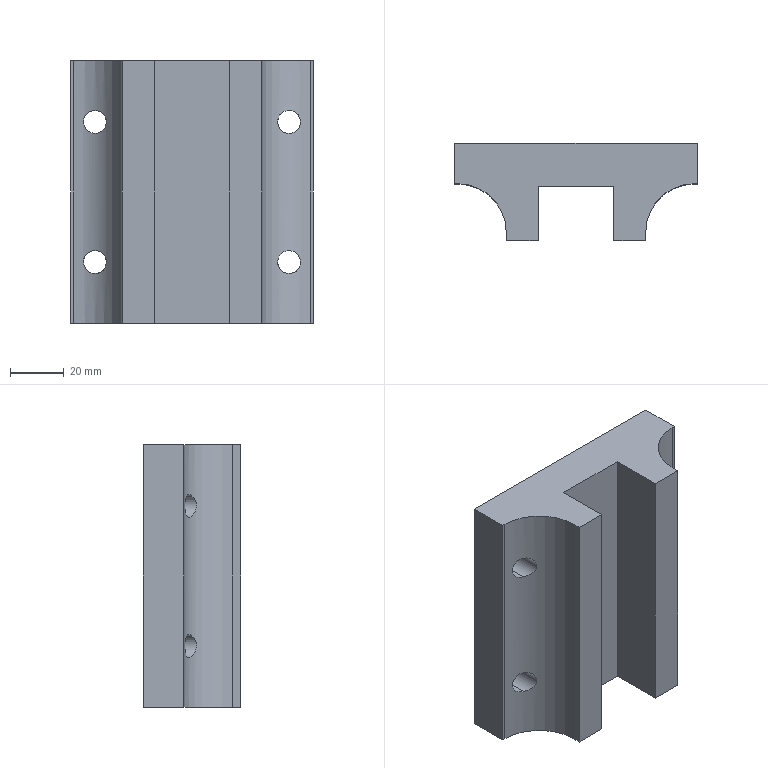Part | SolidWorks | features Extrusion 1, HoleWzd 1 | 1 solid | 24 faces | box 90 x 36 x 97.4 mm | volume 192306 mm3 | plane 14 | cylinder 10 | commonest cylinder face diameters 8.5 x8 36 x2
STEP:
#1=CARTESIAN_POINT('',(36.,-16.792,21.75));
#2=VERTEX_POINT('',#1);
#3=CARTESIAN_POINT('',(36.,-16.792,30.25));
#4=VERTEX_POINT('',#3);
#5=CARTESIAN_POINT('',(36.,-16.792,21.75));
#6=CARTESIAN_POINT('',(35.726,-16.925,21.75));
#7=CARTESIAN_POINT('',(35.454,-17.065,21.776));
#8=CARTESIAN_POINT('',(34.923,-17.356,21.88));
#9=CARTESIAN_POINT('',(34.668,-17.504,21.956));
#10=CARTESIAN_POINT('',(34.176,-17.805,22.152));
#11=CARTESIAN_POINT('',(33.939,-17.959,22.274));
#12=CARTESIAN_POINT('',(33.491,-18.263,22.559));
#13=CARTESIAN_POINT('',(33.282,-18.413,22.722));
#14=CARTESIAN_POINT('',(32.893,-18.702,23.088));
#15=CARTESIAN_POINT('',(32.712,-18.843,23.293));
#16=CARTESIAN_POINT('',(32.388,-19.104,23.744));
#17=CARTESIAN_POINT('',(32.246,-19.222,23.986));
#18=CARTESIAN_POINT('',(32.009,-19.425,24.512));
#19=CARTESIAN_POINT('',(31.913,-19.51,24.796));
#20=CARTESIAN_POINT('',(31.785,-19.624,25.381));
#21=CARTESIAN_POINT('',(31.75,-19.656,25.691));
#22=CARTESIAN_POINT('',(31.75,-19.656,26.148));
#23=CARTESIAN_POINT('',(31.758,-19.649,26.3));
#24=CARTESIAN_POINT('',(31.79,-19.62,26.602));
#25=CARTESIAN_POINT('',(31.815,-19.598,26.754));
#26=CARTESIAN_POINT('',(31.911,-19.512,27.197));
#27=CARTESIAN_POINT('',(32.004,-19.429,27.476));
#28=CARTESIAN_POINT('',(32.243,-19.225,28.008));
#29=CARTESIAN_POINT('',(32.384,-19.107,28.251));
#30=CARTESIAN_POINT('',(32.705,-18.848,28.699));
#31=CARTESIAN_POINT('',(32.887,-18.706,28.906));
#32=CARTESIAN_POINT('',(33.279,-18.415,29.275));
#33=CARTESIAN_POINT('',(33.488,-18.265,29.439));
#34=CARTESIAN_POINT('',(33.936,-17.961,29.725));
#35=CARTESIAN_POINT('',(34.174,-17.806,29.847));
#36=CARTESIAN_POINT('',(34.665,-17.505,30.044));
#37=CARTESIAN_POINT('',(34.92,-17.357,30.119));
#38=CARTESIAN_POINT('',(35.448,-17.068,30.223));
#39=CARTESIAN_POINT('',(35.723,-16.926,30.25));
#40=CARTESIAN_POINT('',(36.,-16.792,30.25));
#41=B_SPLINE_CURVE_WITH_KNOTS('',3,(#5,#6,#7,#8,#9,#10,#11,#12,#13,#14,#15,#16,#17,#18,#19,#20,#21,#22,#23,#24,#25,#26,#27,#28,#29,#30,#31,#32,#33,#34,#35,#36,#37,#38,#39,#40),.UNSPECIFIED.,.F.,.F.,(4,2,2,2,2,2,2,2,2,2,2,2,2,2,2,2,2,4),(0.01371,0.01462,0.01554,0.01645,0.01736,0.01827,0.01918,0.02009,0.02101,0.02146,0.02192,0.02283,0.02374,0.02465,0.02557,0.02648,0.02739,0.0283),.UNSPECIFIED.);
#42=EDGE_CURVE('',#2,#4,#41,.T.);
#43=ORIENTED_EDGE('',*,*,#42,.F.);
#44=CARTESIAN_POINT('',(36.,0.,21.75));
#45=VERTEX_POINT('',#44);
#46=CARTESIAN_POINT('',(36.,0.,21.75));
#47=DIRECTION('',(0.,1.,0.));
#48=VECTOR('',#47,1000.);
#49=LINE('',#46,#48);
#50=EDGE_CURVE('',#2,#45,#49,.T.);
#51=ORIENTED_EDGE('',*,*,#50,.T.);
#52=CARTESIAN_POINT('',(36.,0.,30.25));
#53=VERTEX_POINT('',#52);
#54=CARTESIAN_POINT('',(36.,0.,26.));
#55=DIRECTION('',(0.,1.,0.));
#56=DIRECTION('',(0.,0.,1.));
#57=AXIS2_PLACEMENT_3D('',#54,#55,#56);
#58=CIRCLE('',#57,4.25);
#59=EDGE_CURVE('',#45,#53,#58,.T.);
#60=ORIENTED_EDGE('',*,*,#59,.T.);
#61=CARTESIAN_POINT('',(36.,0.,30.25));
#62=DIRECTION('',(0.,1.,0.));
#63=VECTOR('',#62,1000.);
#64=LINE('',#61,#63);
#65=EDGE_CURVE('',#4,#53,#64,.T.);
#66=ORIENTED_EDGE('',*,*,#65,.F.);
#67=EDGE_LOOP('',(#43,#51,#60,#66));
#68=FACE_OUTER_BOUND('',#67,.T.);
#69=CARTESIAN_POINT('',(36.,0.,26.));
#70=DIRECTION('',(0.,1.,0.));
#71=DIRECTION('',(0.,0.,1.));
#72=AXIS2_PLACEMENT_3D('',#69,#70,#71);
#73=CYLINDRICAL_SURFACE('',#72,4.25);
#74=ADVANCED_FACE('',(#68),#73,.F.);
#75=CARTESIAN_POINT('',(-36.,-16.792,21.75));
#76=VERTEX_POINT('',#75);
#77=CARTESIAN_POINT('',(-36.,-16.792,30.25));
#78=VERTEX_POINT('',#77);
#79=CARTESIAN_POINT('',(-36.,-16.792,21.75));
#80=CARTESIAN_POINT('',(-36.256,-16.669,21.75));
#81=CARTESIAN_POINT('',(-36.515,-16.551,21.773));
#82=CARTESIAN_POINT('',(-37.04,-16.328,21.87));
#83=CARTESIAN_POINT('',(-37.297,-16.225,21.944));
#84=CARTESIAN_POINT('',(-37.798,-16.039,22.14));
#85=CARTESIAN_POINT('',(-38.042,-15.954,22.262));
#86=CARTESIAN_POINT('',(-38.513,-15.801,22.562));
#87=CARTESIAN_POINT('',(-38.734,-15.735,22.734));
#88=CARTESIAN_POINT('',(-39.138,-15.621,23.12));
#89=CARTESIAN_POINT('',(-39.325,-15.572,23.337));
#90=CARTESIAN_POINT('',(-39.651,-15.491,23.806));
#91=CARTESIAN_POINT('',(-39.789,-15.459,24.054));
#92=CARTESIAN_POINT('',(-40.015,-15.409,24.578));
#93=CARTESIAN_POINT('',(-40.103,-15.39,24.857));
#94=CARTESIAN_POINT('',(-40.22,-15.366,25.417));
#95=CARTESIAN_POINT('',(-40.249,-15.36,25.702));
#96=CARTESIAN_POINT('',(-40.251,-15.36,26.28));
#97=CARTESIAN_POINT('',(-40.222,-15.365,26.567));
#98=CARTESIAN_POINT('',(-40.108,-15.389,27.127));
#99=CARTESIAN_POINT('',(-40.021,-15.407,27.405));
#100=CARTESIAN_POINT('',(-39.796,-15.457,27.932));
#101=CARTESIAN_POINT('',(-39.659,-15.489,28.181));
#102=CARTESIAN_POINT('',(-39.336,-15.569,28.649));
#103=CARTESIAN_POINT('',(-39.149,-15.618,28.868));
#104=CARTESIAN_POINT('',(-38.745,-15.732,29.257));
#105=CARTESIAN_POINT('',(-38.525,-15.798,29.43));
#106=CARTESIAN_POINT('',(-38.054,-15.95,29.731));
#107=CARTESIAN_POINT('',(-37.81,-16.035,29.855));
#108=CARTESIAN_POINT('',(-37.306,-16.222,30.053));
#109=CARTESIAN_POINT('',(-37.044,-16.326,30.128));
#110=CARTESIAN_POINT('',(-36.522,-16.548,30.226));
#111=CARTESIAN_POINT('',(-36.261,-16.667,30.25));
#112=CARTESIAN_POINT('',(-36.,-16.792,30.25));
#113=B_SPLINE_CURVE_WITH_KNOTS('',3,(#79,#80,#81,#82,#83,#84,#85,#86,#87,#88,#89,#90,#91,#92,#93,#94,#95,#96,#97,#98,#99,#100,#101,#102,#103,#104,#105,#106,#107,#108,#109,#110,#111,#112),.UNSPECIFIED.,.F.,.F.,(4,2,2,2,2,2,2,2,2,2,2,2,2,2,2,2,4),(0.01459,0.01544,0.0163,0.01715,0.01801,0.01886,0.01972,0.02057,0.02143,0.02228,0.02314,0.02399,0.02485,0.0257,0.02656,0.02741,0.02827),.UNSPECIFIED.);
#114=EDGE_CURVE('',#76,#78,#113,.T.);
#115=ORIENTED_EDGE('',*,*,#114,.F.);
#116=CARTESIAN_POINT('',(-36.,0.,21.75));
#117=VERTEX_POINT('',#116);
#118=CARTESIAN_POINT('',(-36.,0.,21.75));
#119=DIRECTION('',(0.,1.,0.));
#120=VECTOR('',#119,1000.);
#121=LINE('',#118,#120);
#122=EDGE_CURVE('',#76,#117,#121,.T.);
#123=ORIENTED_EDGE('',*,*,#122,.T.);
#124=CARTESIAN_POINT('',(-36.,0.,30.25));
#125=VERTEX_POINT('',#124);
#126=CARTESIAN_POINT('',(-36.,0.,26.));
#127=DIRECTION('',(0.,1.,0.));
#128=DIRECTION('',(0.,0.,1.));
#129=AXIS2_PLACEMENT_3D('',#126,#127,#128);
#130=CIRCLE('',#129,4.25);
#131=EDGE_CURVE('',#117,#125,#130,.T.);
#132=ORIENTED_EDGE('',*,*,#131,.T.);
#133=CARTESIAN_POINT('',(-36.,0.,30.25));
#134=DIRECTION('',(0.,1.,0.));
#135=VECTOR('',#134,1000.);
#136=LINE('',#133,#135);
#137=EDGE_CURVE('',#78,#125,#136,.T.);
#138=ORIENTED_EDGE('',*,*,#137,.F.);
#139=EDGE_LOOP('',(#115,#123,#132,#138));
#140=FACE_OUTER_BOUND('',#139,.T.);
#141=CARTESIAN_POINT('',(-36.,0.,26.));
#142=DIRECTION('',(0.,1.,0.));
#143=DIRECTION('',(0.,0.,1.));
#144=AXIS2_PLACEMENT_3D('',#141,#142,#143);
#145=CYLINDRICAL_SURFACE('',#144,4.25);
#146=ADVANCED_FACE('',(#140),#145,.F.);
#147=CARTESIAN_POINT('',(36.,-16.792,-30.25));
#148=VERTEX_POINT('',#147);
#149=CARTESIAN_POINT('',(36.,-16.792,-21.75));
#150=VERTEX_POINT('',#149);
#151=CARTESIAN_POINT('',(36.,-16.792,-30.25));
#152=CARTESIAN_POINT('',(35.726,-16.925,-30.25));
#153=CARTESIAN_POINT('',(35.454,-17.065,-30.224));
#154=CARTESIAN_POINT('',(34.923,-17.356,-30.12));
#155=CARTESIAN_POINT('',(34.668,-17.504,-30.044));
#156=CARTESIAN_POINT('',(34.176,-17.805,-29.848));
#157=CARTESIAN_POINT('',(33.939,-17.959,-29.726));
#158=CARTESIAN_POINT('',(33.491,-18.263,-29.441));
#159=CARTESIAN_POINT('',(33.282,-18.413,-29.278));
#160=CARTESIAN_POINT('',(32.893,-18.702,-28.912));
#161=CARTESIAN_POINT('',(32.712,-18.843,-28.707));
#162=CARTESIAN_POINT('',(32.388,-19.104,-28.256));
#163=CARTESIAN_POINT('',(32.246,-19.222,-28.014));
#164=CARTESIAN_POINT('',(32.009,-19.425,-27.488));
#165=CARTESIAN_POINT('',(31.913,-19.51,-27.204));
#166=CARTESIAN_POINT('',(31.785,-19.624,-26.619));
#167=CARTESIAN_POINT('',(31.75,-19.656,-26.309));
#168=CARTESIAN_POINT('',(31.75,-19.656,-25.852));
#169=CARTESIAN_POINT('',(31.758,-19.649,-25.7));
#170=CARTESIAN_POINT('',(31.79,-19.62,-25.398));
#171=CARTESIAN_POINT('',(31.815,-19.598,-25.246));
#172=CARTESIAN_POINT('',(31.911,-19.512,-24.803));
#173=CARTESIAN_POINT('',(32.004,-19.429,-24.524));
#174=CARTESIAN_POINT('',(32.243,-19.225,-23.992));
#175=CARTESIAN_POINT('',(32.384,-19.107,-23.749));
#176=CARTESIAN_POINT('',(32.705,-18.848,-23.301));
#177=CARTESIAN_POINT('',(32.887,-18.706,-23.094));
#178=CARTESIAN_POINT('',(33.279,-18.415,-22.725));
#179=CARTESIAN_POINT('',(33.488,-18.265,-22.561));
#180=CARTESIAN_POINT('',(33.936,-17.961,-22.275));
#181=CARTESIAN_POINT('',(34.174,-17.806,-22.153));
#182=CARTESIAN_POINT('',(34.665,-17.505,-21.956));
#183=CARTESIAN_POINT('',(34.92,-17.357,-21.881));
#184=CARTESIAN_POINT('',(35.448,-17.068,-21.777));
#185=CARTESIAN_POINT('',(35.723,-16.926,-21.75));
#186=CARTESIAN_POINT('',(36.,-16.792,-21.75));
#187=B_SPLINE_CURVE_WITH_KNOTS('',3,(#151,#152,#153,#154,#155,#156,#157,#158,#159,#160,#161,#162,#163,#164,#165,#166,#167,#168,#169,#170,#171,#172,#173,#174,#175,#176,#177,#178,#179,#180,#181,#182,#183,#184,#185,#186),.UNSPECIFIED.,.F.,.F.,(4,2,2,2,2,2,2,2,2,2,2,2,2,2,2,2,2,4),(0.01371,0.01462,0.01554,0.01645,0.01736,0.01827,0.01918,0.02009,0.02101,0.02146,0.02192,0.02283,0.02374,0.02465,0.02557,0.02648,0.02739,0.0283),.UNSPECIFIED.);
#188=EDGE_CURVE('',#148,#150,#187,.T.);
#189=ORIENTED_EDGE('',*,*,#188,.F.);
#190=CARTESIAN_POINT('',(36.,0.,-30.25));
#191=VERTEX_POINT('',#190);
#192=CARTESIAN_POINT('',(36.,0.,-30.25));
#193=DIRECTION('',(0.,1.,0.));
#194=VECTOR('',#193,1000.);
#195=LINE('',#192,#194);
#196=EDGE_CURVE('',#148,#191,#195,.T.);
#197=ORIENTED_EDGE('',*,*,#196,.T.);
#198=CARTESIAN_POINT('',(36.,0.,-21.75));
#199=VERTEX_POINT('',#198);
#200=CARTESIAN_POINT('',(36.,0.,-26.));
#201=DIRECTION('',(0.,1.,0.));
#202=DIRECTION('',(0.,0.,1.));
#203=AXIS2_PLACEMENT_3D('',#200,#201,#202);
#204=CIRCLE('',#203,4.25);
#205=EDGE_CURVE('',#191,#199,#204,.T.);
#206=ORIENTED_EDGE('',*,*,#205,.T.);
#207=CARTESIAN_POINT('',(36.,0.,-21.75));
#208=DIRECTION('',(0.,1.,0.));
#209=VECTOR('',#208,1000.);
#210=LINE('',#207,#209);
#211=EDGE_CURVE('',#150,#199,#210,.T.);
#212=ORIENTED_EDGE('',*,*,#211,.F.);
#213=EDGE_LOOP('',(#189,#197,#206,#212));
#214=FACE_OUTER_BOUND('',#213,.T.);
#215=CARTESIAN_POINT('',(36.,0.,-26.));
#216=DIRECTION('',(0.,1.,0.));
#217=DIRECTION('',(0.,0.,1.));
#218=AXIS2_PLACEMENT_3D('',#215,#216,#217);
#219=CYLINDRICAL_SURFACE('',#218,4.25);
#220=ADVANCED_FACE('',(#214),#219,.F.);
#221=CARTESIAN_POINT('',(-36.,-16.792,-30.25));
#222=VERTEX_POINT('',#221);
#223=CARTESIAN_POINT('',(-36.,-16.792,-21.75));
#224=VERTEX_POINT('',#223);
#225=CARTESIAN_POINT('',(-36.,-16.792,-30.25));
#226=CARTESIAN_POINT('',(-36.256,-16.669,-30.25));
#227=CARTESIAN_POINT('',(-36.515,-16.551,-30.227));
#228=CARTESIAN_POINT('',(-37.04,-16.328,-30.13));
#229=CARTESIAN_POINT('',(-37.297,-16.225,-30.056));
#230=CARTESIAN_POINT('',(-37.798,-16.039,-29.86));
#231=CARTESIAN_POINT('',(-38.042,-15.954,-29.738));
#232=CARTESIAN_POINT('',(-38.513,-15.801,-29.438));
#233=CARTESIAN_POINT('',(-38.734,-15.735,-29.266));
#234=CARTESIAN_POINT('',(-39.138,-15.621,-28.88));
#235=CARTESIAN_POINT('',(-39.325,-15.572,-28.663));
#236=CARTESIAN_POINT('',(-39.651,-15.491,-28.194));
#237=CARTESIAN_POINT('',(-39.789,-15.459,-27.946));
#238=CARTESIAN_POINT('',(-40.015,-15.409,-27.422));
#239=CARTESIAN_POINT('',(-40.103,-15.39,-27.143));
#240=CARTESIAN_POINT('',(-40.22,-15.366,-26.583));
#241=CARTESIAN_POINT('',(-40.249,-15.36,-26.298));
#242=CARTESIAN_POINT('',(-40.251,-15.36,-25.72));
#243=CARTESIAN_POINT('',(-40.222,-15.365,-25.433));
#244=CARTESIAN_POINT('',(-40.108,-15.389,-24.873));
#245=CARTESIAN_POINT('',(-40.021,-15.407,-24.595));
#246=CARTESIAN_POINT('',(-39.796,-15.457,-24.068));
#247=CARTESIAN_POINT('',(-39.659,-15.489,-23.819));
#248=CARTESIAN_POINT('',(-39.336,-15.569,-23.351));
#249=CARTESIAN_POINT('',(-39.149,-15.618,-23.132));
#250=CARTESIAN_POINT('',(-38.745,-15.732,-22.743));
#251=CARTESIAN_POINT('',(-38.525,-15.798,-22.57));
#252=CARTESIAN_POINT('',(-38.054,-15.95,-22.269));
#253=CARTESIAN_POINT('',(-37.81,-16.035,-22.145));
#254=CARTESIAN_POINT('',(-37.306,-16.222,-21.947));
#255=CARTESIAN_POINT('',(-37.044,-16.326,-21.872));
#256=CARTESIAN_POINT('',(-36.522,-16.548,-21.774));
#257=CARTESIAN_POINT('',(-36.261,-16.667,-21.75));
#258=CARTESIAN_POINT('',(-36.,-16.792,-21.75));
#259=B_SPLINE_CURVE_WITH_KNOTS('',3,(#225,#226,#227,#228,#229,#230,#231,#232,#233,#234,#235,#236,#237,#238,#239,#240,#241,#242,#243,#244,#245,#246,#247,#248,#249,#250,#251,#252,#253,#254,#255,#256,#257,#258),.UNSPECIFIED.,.F.,.F.,(4,2,2,2,2,2,2,2,2,2,2,2,2,2,2,2,4),(0.01459,0.01544,0.0163,0.01715,0.01801,0.01886,0.01972,0.02057,0.02143,0.02228,0.02314,0.02399,0.02485,0.0257,0.02656,0.02741,0.02827),.UNSPECIFIED.);
#260=EDGE_CURVE('',#222,#224,#259,.T.);
#261=ORIENTED_EDGE('',*,*,#260,.F.);
#262=CARTESIAN_POINT('',(-36.,0.,-30.25));
#263=VERTEX_POINT('',#262);
#264=CARTESIAN_POINT('',(-36.,0.,-30.25));
#265=DIRECTION('',(0.,1.,0.));
#266=VECTOR('',#265,1000.);
#267=LINE('',#264,#266);
#268=EDGE_CURVE('',#222,#263,#267,.T.);
#269=ORIENTED_EDGE('',*,*,#268,.T.);
#270=CARTESIAN_POINT('',(-36.,0.,-21.75));
#271=VERTEX_POINT('',#270);
#272=CARTESIAN_POINT('',(-36.,0.,-26.));
#273=DIRECTION('',(0.,1.,0.));
#274=DIRECTION('',(0.,0.,1.));
#275=AXIS2_PLACEMENT_3D('',#272,#273,#274);
#276=CIRCLE('',#275,4.25);
#277=EDGE_CURVE('',#263,#271,#276,.T.);
#278=ORIENTED_EDGE('',*,*,#277,.T.);
#279=CARTESIAN_POINT('',(-36.,0.,-21.75));
#280=DIRECTION('',(0.,1.,0.));
#281=VECTOR('',#280,1000.);
#282=LINE('',#279,#281);
#283=EDGE_CURVE('',#224,#271,#282,.T.);
#284=ORIENTED_EDGE('',*,*,#283,.F.);
#285=EDGE_LOOP('',(#261,#269,#278,#284));
#286=FACE_OUTER_BOUND('',#285,.T.);
#287=CARTESIAN_POINT('',(-36.,0.,-26.));
#288=DIRECTION('',(0.,1.,0.));
#289=DIRECTION('',(0.,0.,1.));
#290=AXIS2_PLACEMENT_3D('',#287,#288,#289);
#291=CYLINDRICAL_SURFACE('',#290,4.25);
#292=ADVANCED_FACE('',(#286),#291,.F.);
#293=CARTESIAN_POINT('',(-25.83,-36.,-48.7));
#294=VERTEX_POINT('',#293);
#295=CARTESIAN_POINT('',(-14.,-36.,-48.7));
#296=VERTEX_POINT('',#295);
#297=CARTESIAN_POINT('',(-14.,-36.,-48.7));
#298=DIRECTION('',(1.,0.,0.));
#299=VECTOR('',#298,1000.);
#300=LINE('',#297,#299);
#301=EDGE_CURVE('',#294,#296,#300,.T.);
#302=ORIENTED_EDGE('',*,*,#301,.T.);
#303=CARTESIAN_POINT('',(-14.,-36.,48.7));
#304=VERTEX_POINT('',#303);
#305=CARTESIAN_POINT('',(-14.,-36.,48.7));
#306=DIRECTION('',(0.,0.,-1.));
#307=VECTOR('',#306,1000.);
#308=LINE('',#305,#307);
#309=EDGE_CURVE('',#304,#296,#308,.T.);
#310=ORIENTED_EDGE('',*,*,#309,.F.);
#311=CARTESIAN_POINT('',(-25.83,-36.,48.7));
#312=VERTEX_POINT('',#311);
#313=CARTESIAN_POINT('',(-14.,-36.,48.7));
#314=DIRECTION('',(1.,0.,0.));
#315=VECTOR('',#314,1000.);
#316=LINE('',#313,#315);
#317=EDGE_CURVE('',#312,#304,#316,.T.);
#318=ORIENTED_EDGE('',*,*,#317,.F.);
#319=CARTESIAN_POINT('',(-25.83,-36.,48.7));
#320=DIRECTION('',(0.,0.,-1.));
#321=VECTOR('',#320,1000.);
#322=LINE('',#319,#321);
#323=EDGE_CURVE('',#312,#294,#322,.T.);
#324=ORIENTED_EDGE('',*,*,#323,.T.);
#325=EDGE_LOOP('',(#302,#310,#318,#324));
#326=FACE_OUTER_BOUND('',#325,.T.);
#327=CARTESIAN_POINT('',(-14.,-36.,48.7));
#328=DIRECTION('',(0.,1.,0.));
#329=DIRECTION('',(0.,0.,1.));
#330=AXIS2_PLACEMENT_3D('',#327,#328,#329);
#331=PLANE('',#330);
#332=ADVANCED_FACE('',(#326),#331,.F.);
#333=CARTESIAN_POINT('',(-14.,-16.,-48.7));
#334=VERTEX_POINT('',#333);
#335=CARTESIAN_POINT('',(-14.,-36.,-48.7));
#336=DIRECTION('',(0.,1.,0.));
#337=VECTOR('',#336,1000.);
#338=LINE('',#335,#337);
#339=EDGE_CURVE('',#296,#334,#338,.T.);
#340=ORIENTED_EDGE('',*,*,#339,.T.);
#341=CARTESIAN_POINT('',(-14.,-16.,48.7));
#342=VERTEX_POINT('',#341);
#343=CARTESIAN_POINT('',(-14.,-16.,48.7));
#344=DIRECTION('',(0.,0.,-1.));
#345=VECTOR('',#344,1000.);
#346=LINE('',#343,#345);
#347=EDGE_CURVE('',#342,#334,#346,.T.);
#348=ORIENTED_EDGE('',*,*,#347,.F.);
#349=CARTESIAN_POINT('',(-14.,-36.,48.7));
#350=DIRECTION('',(0.,1.,0.));
#351=VECTOR('',#350,1000.);
#352=LINE('',#349,#351);
#353=EDGE_CURVE('',#304,#342,#352,.T.);
#354=ORIENTED_EDGE('',*,*,#353,.F.);
#355=ORIENTED_EDGE('',*,*,#309,.T.);
#356=EDGE_LOOP('',(#340,#348,#354,#355));
#357=FACE_OUTER_BOUND('',#356,.T.);
#358=CARTESIAN_POINT('',(-14.,-36.,48.7));
#359=DIRECTION('',(-1.,0.,0.));
#360=DIRECTION('',(0.,0.,1.));
#361=AXIS2_PLACEMENT_3D('',#358,#359,#360);
#362=PLANE('',#361);
#363=ADVANCED_FACE('',(#357),#362,.F.);
#364=CARTESIAN_POINT('',(14.,-16.,-48.7));
#365=VERTEX_POINT('',#364);
#366=CARTESIAN_POINT('',(-14.,-16.,-48.7));
#367=DIRECTION('',(1.,0.,0.));
#368=VECTOR('',#367,1000.);
#369=LINE('',#366,#368);
#370=EDGE_CURVE('',#334,#365,#369,.T.);
#371=ORIENTED_EDGE('',*,*,#370,.T.);
#372=CARTESIAN_POINT('',(14.,-16.,48.7));
#373=VERTEX_POINT('',#372);
#374=CARTESIAN_POINT('',(14.,-16.,48.7));
#375=DIRECTION('',(0.,0.,-1.));
#376=VECTOR('',#375,1000.);
#377=LINE('',#374,#376);
#378=EDGE_CURVE('',#373,#365,#377,.T.);
#379=ORIENTED_EDGE('',*,*,#378,.F.);
#380=CARTESIAN_POINT('',(-14.,-16.,48.7));
#381=DIRECTION('',(1.,0.,0.));
#382=VECTOR('',#381,1000.);
#383=LINE('',#380,#382);
#384=EDGE_CURVE('',#342,#373,#383,.T.);
#385=ORIENTED_EDGE('',*,*,#384,.F.);
#386=ORIENTED_EDGE('',*,*,#347,.T.);
#387=EDGE_LOOP('',(#371,#379,#385,#386));
#388=FACE_OUTER_BOUND('',#387,.T.);
#389=CARTESIAN_POINT('',(-14.,-16.,48.7));
#390=DIRECTION('',(0.,1.,0.));
#391=DIRECTION('',(0.,0.,1.));
#392=AXIS2_PLACEMENT_3D('',#389,#390,#391);
#393=PLANE('',#392);
#394=ADVANCED_FACE('',(#388),#393,.F.);
#395=CARTESIAN_POINT('',(14.,-36.,-48.7));
#396=VERTEX_POINT('',#395);
#397=CARTESIAN_POINT('',(14.,-16.,-48.7));
#398=DIRECTION('',(0.,-1.,0.));
#399=VECTOR('',#398,1000.);
#400=LINE('',#397,#399);
#401=EDGE_CURVE('',#365,#396,#400,.T.);
#402=ORIENTED_EDGE('',*,*,#401,.T.);
#403=CARTESIAN_POINT('',(14.,-36.,48.7));
#404=VERTEX_POINT('',#403);
#405=CARTESIAN_POINT('',(14.,-36.,48.7));
#406=DIRECTION('',(0.,0.,-1.));
#407=VECTOR('',#406,1000.);
#408=LINE('',#405,#407);
#409=EDGE_CURVE('',#404,#396,#408,.T.);
#410=ORIENTED_EDGE('',*,*,#409,.F.);
#411=CARTESIAN_POINT('',(14.,-16.,48.7));
#412=DIRECTION('',(0.,-1.,0.));
#413=VECTOR('',#412,1000.);
#414=LINE('',#411,#413);
#415=EDGE_CURVE('',#373,#404,#414,.T.);
#416=ORIENTED_EDGE('',*,*,#415,.F.);
#417=ORIENTED_EDGE('',*,*,#378,.T.);
#418=EDGE_LOOP('',(#402,#410,#416,#417));
#419=FACE_OUTER_BOUND('',#418,.T.);
#420=CARTESIAN_POINT('',(14.,-16.,48.7));
#421=DIRECTION('',(1.,0.,0.));
#422=DIRECTION('',(0.,1.,0.));
#423=AXIS2_PLACEMENT_3D('',#420,#421,#422);
#424=PLANE('',#423);
#425=ADVANCED_FACE('',(#419),#424,.F.);
#426=CARTESIAN_POINT('',(25.83,-36.,-48.7));
#427=VERTEX_POINT('',#426);
#428=CARTESIAN_POINT('',(25.83,-36.,-48.7));
#429=DIRECTION('',(1.,0.,0.));
#430=VECTOR('',#429,1000.);
#431=LINE('',#428,#430);
#432=EDGE_CURVE('',#396,#427,#431,.T.);
#433=ORIENTED_EDGE('',*,*,#432,.T.);
#434=CARTESIAN_POINT('',(25.83,-36.,48.7));
#435=VERTEX_POINT('',#434);
#436=CARTESIAN_POINT('',(25.83,-36.,48.7));
#437=DIRECTION('',(0.,0.,-1.));
#438=VECTOR('',#437,1000.);
#439=LINE('',#436,#438);
#440=EDGE_CURVE('',#435,#427,#439,.T.);
#441=ORIENTED_EDGE('',*,*,#440,.F.);
#442=CARTESIAN_POINT('',(25.83,-36.,48.7));
#443=DIRECTION('',(1.,0.,0.));
#444=VECTOR('',#443,1000.);
#445=LINE('',#442,#444);
#446=EDGE_CURVE('',#404,#435,#445,.T.);
#447=ORIENTED_EDGE('',*,*,#446,.F.);
#448=ORIENTED_EDGE('',*,*,#409,.T.);
#449=EDGE_LOOP('',(#433,#441,#447,#448));
#450=FACE_OUTER_BOUND('',#449,.T.);
#451=CARTESIAN_POINT('',(25.83,-36.,48.7));
#452=DIRECTION('',(0.,1.,0.));
#453=DIRECTION('',(-1.,0.,0.));
#454=AXIS2_PLACEMENT_3D('',#451,#452,#453);
#455=PLANE('',#454);
#456=ADVANCED_FACE('',(#450),#455,.F.);
#457=CARTESIAN_POINT('',(25.83,-33.,-48.7));
#458=VERTEX_POINT('',#457);
#459=CARTESIAN_POINT('',(25.83,-33.,-48.7));
#460=DIRECTION('',(0.,1.,0.));
#461=VECTOR('',#460,1000.);
#462=LINE('',#459,#461);
#463=EDGE_CURVE('',#427,#458,#462,.T.);
#464=ORIENTED_EDGE('',*,*,#463,.T.);
#465=CARTESIAN_POINT('',(25.83,-33.,48.7));
#466=VERTEX_POINT('',#465);
#467=CARTESIAN_POINT('',(25.83,-33.,48.7));
#468=DIRECTION('',(0.,0.,-1.));
#469=VECTOR('',#468,1000.);
#470=LINE('',#467,#469);
#471=EDGE_CURVE('',#466,#458,#470,.T.);
#472=ORIENTED_EDGE('',*,*,#471,.F.);
#473=CARTESIAN_POINT('',(25.83,-33.,48.7));
#474=DIRECTION('',(0.,1.,0.));
#475=VECTOR('',#474,1000.);
#476=LINE('',#473,#475);
#477=EDGE_CURVE('',#435,#466,#476,.T.);
#478=ORIENTED_EDGE('',*,*,#477,.F.);
#479=ORIENTED_EDGE('',*,*,#440,.T.);
#480=EDGE_LOOP('',(#464,#472,#478,#479));
#481=FACE_OUTER_BOUND('',#480,.T.);
#482=CARTESIAN_POINT('',(25.83,-33.,48.7));
#483=DIRECTION('',(-1.,0.,0.));
#484=DIRECTION('',(0.,-1.,0.));
#485=AXIS2_PLACEMENT_3D('',#482,#483,#484);
#486=PLANE('',#485);
#487=ADVANCED_FACE('',(#481),#486,.F.);
#488=CARTESIAN_POINT('',(36.,-16.792,30.25));
#489=CARTESIAN_POINT('',(36.261,-16.667,30.25));
#490=CARTESIAN_POINT('',(36.521,-16.549,30.226));
#491=CARTESIAN_POINT('',(37.039,-16.328,30.13));
#492=CARTESIAN_POINT('',(37.299,-16.225,30.056));
#493=CARTESIAN_POINT('',(37.806,-16.036,29.857));
#494=CARTESIAN_POINT('',(38.049,-15.952,29.733));
#495=CARTESIAN_POINT('',(38.514,-15.801,29.438));
#496=CARTESIAN_POINT('',(38.738,-15.734,29.263));
#497=CARTESIAN_POINT('',(39.144,-15.619,28.873));
#498=CARTESIAN_POINT('',(39.327,-15.572,28.66));
#499=CARTESIAN_POINT('',(39.652,-15.491,28.193));
#500=CARTESIAN_POINT('',(39.792,-15.458,27.939));
#501=CARTESIAN_POINT('',(40.017,-15.408,27.416));
#502=CARTESIAN_POINT('',(40.104,-15.39,27.143));
#503=CARTESIAN_POINT('',(40.221,-15.366,26.576));
#504=CARTESIAN_POINT('',(40.25,-15.36,26.291));
#505=CARTESIAN_POINT('',(40.25,-15.36,25.718));
#506=CARTESIAN_POINT('',(40.221,-15.365,25.428));
#507=CARTESIAN_POINT('',(40.106,-15.389,24.866));
#508=CARTESIAN_POINT('',(40.021,-15.407,24.593));
#509=CARTESIAN_POINT('',(39.795,-15.458,24.066));
#510=CARTESIAN_POINT('',(39.655,-15.49,23.813));
#511=CARTESIAN_POINT('',(39.333,-15.57,23.348));
#512=CARTESIAN_POINT('',(39.148,-15.618,23.131));
#513=CARTESIAN_POINT('',(38.74,-15.734,22.739));
#514=CARTESIAN_POINT('',(38.52,-15.799,22.567));
#515=CARTESIAN_POINT('',(38.054,-15.95,22.269));
#516=CARTESIAN_POINT('',(37.805,-16.036,22.143));
#517=CARTESIAN_POINT('',(37.301,-16.224,21.945));
#518=CARTESIAN_POINT('',(37.044,-16.326,21.872));
#519=CARTESIAN_POINT('',(36.521,-16.549,21.774));
#520=CARTESIAN_POINT('',(36.258,-16.668,21.75));
#521=CARTESIAN_POINT('',(36.,-16.792,21.75));
#522=B_SPLINE_CURVE_WITH_KNOTS('',3,(#488,#489,#490,#491,#492,#493,#494,#495,#496,#497,#498,#499,#500,#501,#502,#503,#504,#505,#506,#507,#508,#509,#510,#511,#512,#513,#514,#515,#516,#517,#518,#519,#520,#521),.UNSPECIFIED.,.F.,.F.,(4,2,2,2,2,2,2,2,2,2,2,2,2,2,2,2,4),(0.,0.000857,0.001714,0.002571,0.003428,0.004285,0.005142,0.005999,0.006856,0.007713,0.00857,0.009427,0.01028,0.01114,0.012,0.01285,0.01371),.UNSPECIFIED.);
#523=EDGE_CURVE('',#4,#2,#522,.T.);
#524=ORIENTED_EDGE('',*,*,#523,.T.);
#525=ORIENTED_EDGE('',*,*,#42,.T.);
#526=EDGE_LOOP('',(#524,#525));
#527=FACE_BOUND('',#526,.T.);
#528=CARTESIAN_POINT('',(36.,-16.792,-21.75));
#529=CARTESIAN_POINT('',(36.261,-16.667,-21.75));
#530=CARTESIAN_POINT('',(36.521,-16.549,-21.774));
#531=CARTESIAN_POINT('',(37.039,-16.328,-21.87));
#532=CARTESIAN_POINT('',(37.299,-16.225,-21.944));
#533=CARTESIAN_POINT('',(37.806,-16.036,-22.143));
#534=CARTESIAN_POINT('',(38.049,-15.952,-22.267));
#535=CARTESIAN_POINT('',(38.514,-15.801,-22.562));
#536=CARTESIAN_POINT('',(38.738,-15.734,-22.737));
#537=CARTESIAN_POINT('',(39.144,-15.619,-23.127));
#538=CARTESIAN_POINT('',(39.327,-15.572,-23.34));
#539=CARTESIAN_POINT('',(39.652,-15.491,-23.807));
#540=CARTESIAN_POINT('',(39.792,-15.458,-24.061));
#541=CARTESIAN_POINT('',(40.017,-15.408,-24.584));
#542=CARTESIAN_POINT('',(40.104,-15.39,-24.857));
#543=CARTESIAN_POINT('',(40.221,-15.366,-25.424));
#544=CARTESIAN_POINT('',(40.25,-15.36,-25.709));
#545=CARTESIAN_POINT('',(40.25,-15.36,-26.282));
#546=CARTESIAN_POINT('',(40.221,-15.365,-26.572));
#547=CARTESIAN_POINT('',(40.106,-15.389,-27.134));
#548=CARTESIAN_POINT('',(40.021,-15.407,-27.407));
#549=CARTESIAN_POINT('',(39.795,-15.458,-27.934));
#550=CARTESIAN_POINT('',(39.655,-15.49,-28.187));
#551=CARTESIAN_POINT('',(39.333,-15.57,-28.652));
#552=CARTESIAN_POINT('',(39.148,-15.618,-28.869));
#553=CARTESIAN_POINT('',(38.74,-15.734,-29.261));
#554=CARTESIAN_POINT('',(38.52,-15.799,-29.433));
#555=CARTESIAN_POINT('',(38.054,-15.95,-29.731));
#556=CARTESIAN_POINT('',(37.805,-16.036,-29.857));
#557=CARTESIAN_POINT('',(37.301,-16.224,-30.055));
#558=CARTESIAN_POINT('',(37.044,-16.326,-30.128));
#559=CARTESIAN_POINT('',(36.521,-16.549,-30.226));
#560=CARTESIAN_POINT('',(36.258,-16.668,-30.25));
#561=CARTESIAN_POINT('',(36.,-16.792,-30.25));
#562=B_SPLINE_CURVE_WITH_KNOTS('',3,(#528,#529,#530,#531,#532,#533,#534,#535,#536,#537,#538,#539,#540,#541,#542,#543,#544,#545,#546,#547,#548,#549,#550,#551,#552,#553,#554,#555,#556,#557,#558,#559,#560,#561),.UNSPECIFIED.,.F.,.F.,(4,2,2,2,2,2,2,2,2,2,2,2,2,2,2,2,4),(0.,0.000857,0.001714,0.002571,0.003428,0.004285,0.005142,0.005999,0.006856,0.007713,0.00857,0.009427,0.01028,0.01114,0.012,0.01285,0.01371),.UNSPECIFIED.);
#563=EDGE_CURVE('',#150,#148,#562,.T.);
#564=ORIENTED_EDGE('',*,*,#563,.T.);
#565=ORIENTED_EDGE('',*,*,#188,.T.);
#566=EDGE_LOOP('',(#564,#565));
#567=FACE_BOUND('',#566,.T.);
#568=CARTESIAN_POINT('',(43.83,-15.,-48.7));
#569=VERTEX_POINT('',#568);
#570=CARTESIAN_POINT('',(43.83,-33.,-48.7));
#571=DIRECTION('',(0.,0.,-1.));
#572=DIRECTION('',(1.,0.,0.));
#573=AXIS2_PLACEMENT_3D('',#570,#571,#572);
#574=CIRCLE('',#573,18.);
#575=EDGE_CURVE('',#458,#569,#574,.T.);
#576=ORIENTED_EDGE('',*,*,#575,.T.);
#577=CARTESIAN_POINT('',(43.83,-15.,48.7));
#578=VERTEX_POINT('',#577);
#579=CARTESIAN_POINT('',(43.83,-15.,48.7));
#580=DIRECTION('',(0.,0.,-1.));
#581=VECTOR('',#580,1000.);
#582=LINE('',#579,#581);
#583=EDGE_CURVE('',#578,#569,#582,.T.);
#584=ORIENTED_EDGE('',*,*,#583,.F.);
#585=CARTESIAN_POINT('',(43.83,-33.,48.7));
#586=DIRECTION('',(0.,0.,-1.));
#587=DIRECTION('',(1.,0.,0.));
#588=AXIS2_PLACEMENT_3D('',#585,#586,#587);
#589=CIRCLE('',#588,18.);
#590=EDGE_CURVE('',#466,#578,#589,.T.);
#591=ORIENTED_EDGE('',*,*,#590,.F.);
#592=ORIENTED_EDGE('',*,*,#471,.T.);
#593=EDGE_LOOP('',(#576,#584,#591,#592));
#594=FACE_OUTER_BOUND('',#593,.T.);
#595=CARTESIAN_POINT('',(43.83,-33.,48.7));
#596=DIRECTION('',(0.,0.,-1.));
#597=DIRECTION('',(-1.,0.,0.));
#598=AXIS2_PLACEMENT_3D('',#595,#596,#597);
#599=CYLINDRICAL_SURFACE('',#598,18.);
#600=ADVANCED_FACE('',(#527,#567,#594),#599,.F.);
#601=CARTESIAN_POINT('',(45.,-15.,-48.7));
#602=VERTEX_POINT('',#601);
#603=CARTESIAN_POINT('',(45.,-15.,-48.7));
#604=DIRECTION('',(1.,0.,0.));
#605=VECTOR('',#604,1000.);
#606=LINE('',#603,#605);
#607=EDGE_CURVE('',#569,#602,#606,.T.);
#608=ORIENTED_EDGE('',*,*,#607,.T.);
#609=CARTESIAN_POINT('',(45.,-15.,48.7));
#610=VERTEX_POINT('',#609);
#611=CARTESIAN_POINT('',(45.,-15.,48.7));
#612=DIRECTION('',(0.,0.,-1.));
#613=VECTOR('',#612,1000.);
#614=LINE('',#611,#613);
#615=EDGE_CURVE('',#610,#602,#614,.T.);
#616=ORIENTED_EDGE('',*,*,#615,.F.);
#617=CARTESIAN_POINT('',(45.,-15.,48.7));
#618=DIRECTION('',(1.,0.,0.));
#619=VECTOR('',#618,1000.);
#620=LINE('',#617,#619);
#621=EDGE_CURVE('',#578,#610,#620,.T.);
#622=ORIENTED_EDGE('',*,*,#621,.F.);
#623=ORIENTED_EDGE('',*,*,#583,.T.);
#624=EDGE_LOOP('',(#608,#616,#622,#623));
#625=FACE_OUTER_BOUND('',#624,.T.);
#626=CARTESIAN_POINT('',(45.,-15.,48.7));
#627=DIRECTION('',(0.,1.,0.));
#628=DIRECTION('',(0.,0.,1.));
#629=AXIS2_PLACEMENT_3D('',#626,#627,#628);
#630=PLANE('',#629);
#631=ADVANCED_FACE('',(#625),#630,.F.);
#632=CARTESIAN_POINT('',(45.,0.,-48.7));
#633=VERTEX_POINT('',#632);
#634=CARTESIAN_POINT('',(45.,0.,-48.7));
#635=DIRECTION('',(0.,1.,0.));
#636=VECTOR('',#635,1000.);
#637=LINE('',#634,#636);
#638=EDGE_CURVE('',#602,#633,#637,.T.);
#639=ORIENTED_EDGE('',*,*,#638,.T.);
#640=CARTESIAN_POINT('',(45.,0.,48.7));
#641=VERTEX_POINT('',#640);
#642=CARTESIAN_POINT('',(45.,0.,48.7));
#643=DIRECTION('',(0.,0.,-1.));
#644=VECTOR('',#643,1000.);
#645=LINE('',#642,#644);
#646=EDGE_CURVE('',#641,#633,#645,.T.);
#647=ORIENTED_EDGE('',*,*,#646,.F.);
#648=CARTESIAN_POINT('',(45.,0.,48.7));
#649=DIRECTION('',(0.,1.,0.));
#650=VECTOR('',#649,1000.);
#651=LINE('',#648,#650);
#652=EDGE_CURVE('',#610,#641,#651,.T.);
#653=ORIENTED_EDGE('',*,*,#652,.F.);
#654=ORIENTED_EDGE('',*,*,#615,.T.);
#655=EDGE_LOOP('',(#639,#647,#653,#654));
#656=FACE_OUTER_BOUND('',#655,.T.);
#657=CARTESIAN_POINT('',(45.,0.,48.7));
#658=DIRECTION('',(-1.,0.,0.));
#659=DIRECTION('',(0.,0.,1.));
#660=AXIS2_PLACEMENT_3D('',#657,#658,#659);
#661=PLANE('',#660);
#662=ADVANCED_FACE('',(#656),#661,.F.);
#663=CARTESIAN_POINT('',(36.,0.,26.));
#664=DIRECTION('',(0.,1.,0.));
#665=DIRECTION('',(0.,0.,1.));
#666=AXIS2_PLACEMENT_3D('',#663,#664,#665);
#667=CIRCLE('',#666,4.25);
#668=EDGE_CURVE('',#53,#45,#667,.T.);
#669=ORIENTED_EDGE('',*,*,#668,.F.);
#670=ORIENTED_EDGE('',*,*,#59,.F.);
#671=EDGE_LOOP('',(#669,#670));
#672=FACE_BOUND('',#671,.T.);
#673=CARTESIAN_POINT('',(-36.,0.,26.));
#674=DIRECTION('',(0.,1.,0.));
#675=DIRECTION('',(0.,0.,1.));
#676=AXIS2_PLACEMENT_3D('',#673,#674,#675);
#677=CIRCLE('',#676,4.25);
#678=EDGE_CURVE('',#125,#117,#677,.T.);
#679=ORIENTED_EDGE('',*,*,#678,.F.);
#680=ORIENTED_EDGE('',*,*,#131,.F.);
#681=EDGE_LOOP('',(#679,#680));
#682=FACE_BOUND('',#681,.T.);
#683=CARTESIAN_POINT('',(36.,0.,-26.));
#684=DIRECTION('',(0.,1.,0.));
#685=DIRECTION('',(0.,0.,1.));
#686=AXIS2_PLACEMENT_3D('',#683,#684,#685);
#687=CIRCLE('',#686,4.25);
#688=EDGE_CURVE('',#199,#191,#687,.T.);
#689=ORIENTED_EDGE('',*,*,#688,.F.);
#690=ORIENTED_EDGE('',*,*,#205,.F.);
#691=EDGE_LOOP('',(#689,#690));
#692=FACE_BOUND('',#691,.T.);
#693=CARTESIAN_POINT('',(-36.,0.,-26.));
#694=DIRECTION('',(0.,1.,0.));
#695=DIRECTION('',(0.,0.,1.));
#696=AXIS2_PLACEMENT_3D('',#693,#694,#695);
#697=CIRCLE('',#696,4.25);
#698=EDGE_CURVE('',#271,#263,#697,.T.);
#699=ORIENTED_EDGE('',*,*,#698,.F.);
#700=ORIENTED_EDGE('',*,*,#277,.F.);
#701=EDGE_LOOP('',(#699,#700));
#702=FACE_BOUND('',#701,.T.);
#703=CARTESIAN_POINT('',(-45.,0.,-48.7));
#704=VERTEX_POINT('',#703);
#705=CARTESIAN_POINT('',(-45.,0.,-48.7));
#706=DIRECTION('',(-1.,0.,0.));
#707=VECTOR('',#706,1000.);
#708=LINE('',#705,#707);
#709=EDGE_CURVE('',#633,#704,#708,.T.);
#710=ORIENTED_EDGE('',*,*,#709,.T.);
#711=CARTESIAN_POINT('',(-45.,0.,48.7));
#712=VERTEX_POINT('',#711);
#713=CARTESIAN_POINT('',(-45.,0.,48.7));
#714=DIRECTION('',(0.,0.,-1.));
#715=VECTOR('',#714,1000.);
#716=LINE('',#713,#715);
#717=EDGE_CURVE('',#712,#704,#716,.T.);
#718=ORIENTED_EDGE('',*,*,#717,.F.);
#719=CARTESIAN_POINT('',(-45.,0.,48.7));
#720=DIRECTION('',(-1.,0.,0.));
#721=VECTOR('',#720,1000.);
#722=LINE('',#719,#721);
#723=EDGE_CURVE('',#641,#712,#722,.T.);
#724=ORIENTED_EDGE('',*,*,#723,.F.);
#725=ORIENTED_EDGE('',*,*,#646,.T.);
#726=EDGE_LOOP('',(#710,#718,#724,#725));
#727=FACE_OUTER_BOUND('',#726,.T.);
#728=CARTESIAN_POINT('',(-45.,0.,48.7));
#729=DIRECTION('',(0.,-1.,0.));
#730=DIRECTION('',(0.,0.,-1.));
#731=AXIS2_PLACEMENT_3D('',#728,#729,#730);
#732=PLANE('',#731);
#733=ADVANCED_FACE('',(#672,#682,#692,#702,#727),#732,.F.);
#734=CARTESIAN_POINT('',(-45.,-15.,-48.7));
#735=VERTEX_POINT('',#734);
#736=CARTESIAN_POINT('',(-45.,-15.,-48.7));
#737=DIRECTION('',(0.,-1.,0.));
#738=VECTOR('',#737,1000.);
#739=LINE('',#736,#738);
#740=EDGE_CURVE('',#704,#735,#739,.T.);
#741=ORIENTED_EDGE('',*,*,#740,.T.);
#742=CARTESIAN_POINT('',(-45.,-15.,48.7));
#743=VERTEX_POINT('',#742);
#744=CARTESIAN_POINT('',(-45.,-15.,48.7));
#745=DIRECTION('',(0.,0.,-1.));
#746=VECTOR('',#745,1000.);
#747=LINE('',#744,#746);
#748=EDGE_CURVE('',#743,#735,#747,.T.);
#749=ORIENTED_EDGE('',*,*,#748,.F.);
#750=CARTESIAN_POINT('',(-45.,-15.,48.7));
#751=DIRECTION('',(0.,-1.,0.));
#752=VECTOR('',#751,1000.);
#753=LINE('',#750,#752);
#754=EDGE_CURVE('',#712,#743,#753,.T.);
#755=ORIENTED_EDGE('',*,*,#754,.F.);
#756=ORIENTED_EDGE('',*,*,#717,.T.);
#757=EDGE_LOOP('',(#741,#749,#755,#756));
#758=FACE_OUTER_BOUND('',#757,.T.);
#759=CARTESIAN_POINT('',(-45.,-15.,48.7));
#760=DIRECTION('',(1.,0.,0.));
#761=DIRECTION('',(0.,0.,-1.));
#762=AXIS2_PLACEMENT_3D('',#759,#760,#761);
#763=PLANE('',#762);
#764=ADVANCED_FACE('',(#758),#763,.F.);
#765=CARTESIAN_POINT('',(-43.83,-15.,-48.7));
#766=VERTEX_POINT('',#765);
#767=CARTESIAN_POINT('',(-45.,-15.,-48.7));
#768=DIRECTION('',(1.,0.,0.));
#769=VECTOR('',#768,1000.);
#770=LINE('',#767,#769);
#771=EDGE_CURVE('',#735,#766,#770,.T.);
#772=ORIENTED_EDGE('',*,*,#771,.T.);
#773=CARTESIAN_POINT('',(-43.83,-15.,48.7));
#774=VERTEX_POINT('',#773);
#775=CARTESIAN_POINT('',(-43.83,-15.,48.7));
#776=DIRECTION('',(0.,0.,-1.));
#777=VECTOR('',#776,1000.);
#778=LINE('',#775,#777);
#779=EDGE_CURVE('',#774,#766,#778,.T.);
#780=ORIENTED_EDGE('',*,*,#779,.F.);
#781=CARTESIAN_POINT('',(-45.,-15.,48.7));
#782=DIRECTION('',(1.,0.,0.));
#783=VECTOR('',#782,1000.);
#784=LINE('',#781,#783);
#785=EDGE_CURVE('',#743,#774,#784,.T.);
#786=ORIENTED_EDGE('',*,*,#785,.F.);
#787=ORIENTED_EDGE('',*,*,#748,.T.);
#788=EDGE_LOOP('',(#772,#780,#786,#787));
#789=FACE_OUTER_BOUND('',#788,.T.);
#790=CARTESIAN_POINT('',(-45.,-15.,48.7));
#791=DIRECTION('',(0.,1.,0.));
#792=DIRECTION('',(0.,0.,1.));
#793=AXIS2_PLACEMENT_3D('',#790,#791,#792);
#794=PLANE('',#793);
#795=ADVANCED_FACE('',(#789),#794,.F.);
#796=CARTESIAN_POINT('',(-36.,-16.792,30.25));
#797=CARTESIAN_POINT('',(-35.444,-17.061,30.25));
#798=CARTESIAN_POINT('',(-34.919,-17.35,30.145));
#799=CARTESIAN_POINT('',(-33.925,-17.959,29.748));
#800=CARTESIAN_POINT('',(-33.48,-18.265,29.465));
#801=CARTESIAN_POINT('',(-32.889,-18.705,28.908));
#802=CARTESIAN_POINT('',(-32.71,-18.845,28.704));
#803=CARTESIAN_POINT('',(-32.468,-19.039,28.368));
#804=CARTESIAN_POINT('',(-32.392,-19.101,28.251));
#805=CARTESIAN_POINT('',(-32.25,-19.219,28.006));
#806=CARTESIAN_POINT('',(-32.184,-19.275,27.877));
#807=CARTESIAN_POINT('',(-32.006,-19.427,27.482));
#808=CARTESIAN_POINT('',(-31.913,-19.51,27.203));
#809=CARTESIAN_POINT('',(-31.783,-19.626,26.61));
#810=CARTESIAN_POINT('',(-31.75,-19.656,26.308));
#811=CARTESIAN_POINT('',(-31.75,-19.656,25.85));
#812=CARTESIAN_POINT('',(-31.758,-19.649,25.695));
#813=CARTESIAN_POINT('',(-31.791,-19.619,25.39));
#814=CARTESIAN_POINT('',(-31.816,-19.597,25.241));
#815=CARTESIAN_POINT('',(-31.912,-19.511,24.801));
#816=CARTESIAN_POINT('',(-32.007,-19.427,24.515));
#817=CARTESIAN_POINT('',(-32.244,-19.224,23.99));
#818=CARTESIAN_POINT('',(-32.386,-19.105,23.747));
#819=CARTESIAN_POINT('',(-32.711,-18.843,23.294));
#820=CARTESIAN_POINT('',(-32.891,-18.703,23.09));
#821=CARTESIAN_POINT('',(-33.281,-18.413,22.723));
#822=CARTESIAN_POINT('',(-33.491,-18.263,22.559));
#823=CARTESIAN_POINT('',(-33.942,-17.957,22.272));
#824=CARTESIAN_POINT('',(-34.177,-17.805,22.152));
#825=CARTESIAN_POINT('',(-34.668,-17.503,21.955));
#826=CARTESIAN_POINT('',(-34.925,-17.354,21.879));
#827=CARTESIAN_POINT('',(-35.457,-17.063,21.776));
#828=CARTESIAN_POINT('',(-35.727,-16.924,21.75));
#829=CARTESIAN_POINT('',(-36.,-16.792,21.75));
#830=B_SPLINE_CURVE_WITH_KNOTS('',3,(#796,#797,#798,#799,#800,#801,#802,#803,#804,#805,#806,#807,#808,#809,#810,#811,#812,#813,#814,#815,#816,#817,#818,#819,#820,#821,#822,#823,#824,#825,#826,#827,#828,#829),.UNSPECIFIED.,.F.,.F.,(4,2,2,2,2,2,2,2,2,2,2,2,2,2,2,2,4),(0.,0.001823,0.003647,0.004558,0.005014,0.00547,0.006382,0.007293,0.007749,0.008205,0.009117,0.01003,0.01094,0.01185,0.01276,0.01368,0.01459),.UNSPECIFIED.);
#831=EDGE_CURVE('',#78,#76,#830,.T.);
#832=ORIENTED_EDGE('',*,*,#831,.T.);
#833=ORIENTED_EDGE('',*,*,#114,.T.);
#834=EDGE_LOOP('',(#832,#833));
#835=FACE_BOUND('',#834,.T.);
#836=CARTESIAN_POINT('',(-36.,-16.792,-21.75));
#837=CARTESIAN_POINT('',(-35.444,-17.061,-21.75));
#838=CARTESIAN_POINT('',(-34.919,-17.35,-21.855));
#839=CARTESIAN_POINT('',(-33.925,-17.959,-22.252));
#840=CARTESIAN_POINT('',(-33.48,-18.265,-22.535));
#841=CARTESIAN_POINT('',(-32.889,-18.705,-23.092));
#842=CARTESIAN_POINT('',(-32.71,-18.845,-23.296));
#843=CARTESIAN_POINT('',(-32.468,-19.039,-23.632));
#844=CARTESIAN_POINT('',(-32.392,-19.101,-23.749));
#845=CARTESIAN_POINT('',(-32.25,-19.219,-23.994));
#846=CARTESIAN_POINT('',(-32.184,-19.275,-24.123));
#847=CARTESIAN_POINT('',(-32.006,-19.427,-24.518));
#848=CARTESIAN_POINT('',(-31.913,-19.51,-24.797));
#849=CARTESIAN_POINT('',(-31.783,-19.626,-25.39));
#850=CARTESIAN_POINT('',(-31.75,-19.656,-25.692));
#851=CARTESIAN_POINT('',(-31.75,-19.656,-26.15));
#852=CARTESIAN_POINT('',(-31.758,-19.649,-26.305));
#853=CARTESIAN_POINT('',(-31.791,-19.619,-26.61));
#854=CARTESIAN_POINT('',(-31.816,-19.597,-26.759));
#855=CARTESIAN_POINT('',(-31.912,-19.511,-27.199));
#856=CARTESIAN_POINT('',(-32.007,-19.427,-27.485));
#857=CARTESIAN_POINT('',(-32.244,-19.224,-28.01));
#858=CARTESIAN_POINT('',(-32.386,-19.105,-28.253));
#859=CARTESIAN_POINT('',(-32.711,-18.843,-28.706));
#860=CARTESIAN_POINT('',(-32.891,-18.703,-28.91));
#861=CARTESIAN_POINT('',(-33.281,-18.413,-29.277));
#862=CARTESIAN_POINT('',(-33.491,-18.263,-29.441));
#863=CARTESIAN_POINT('',(-33.942,-17.957,-29.728));
#864=CARTESIAN_POINT('',(-34.177,-17.805,-29.848));
#865=CARTESIAN_POINT('',(-34.668,-17.503,-30.045));
#866=CARTESIAN_POINT('',(-34.925,-17.354,-30.121));
#867=CARTESIAN_POINT('',(-35.457,-17.063,-30.224));
#868=CARTESIAN_POINT('',(-35.727,-16.924,-30.25));
#869=CARTESIAN_POINT('',(-36.,-16.792,-30.25));
#870=B_SPLINE_CURVE_WITH_KNOTS('',3,(#836,#837,#838,#839,#840,#841,#842,#843,#844,#845,#846,#847,#848,#849,#850,#851,#852,#853,#854,#855,#856,#857,#858,#859,#860,#861,#862,#863,#864,#865,#866,#867,#868,#869),.UNSPECIFIED.,.F.,.F.,(4,2,2,2,2,2,2,2,2,2,2,2,2,2,2,2,4),(0.,0.001823,0.003647,0.004558,0.005014,0.00547,0.006382,0.007293,0.007749,0.008205,0.009117,0.01003,0.01094,0.01185,0.01276,0.01368,0.01459),.UNSPECIFIED.);
#871=EDGE_CURVE('',#224,#222,#870,.T.);
#872=ORIENTED_EDGE('',*,*,#871,.T.);
#873=ORIENTED_EDGE('',*,*,#260,.T.);
#874=EDGE_LOOP('',(#872,#873));
#875=FACE_BOUND('',#874,.T.);
#876=CARTESIAN_POINT('',(-25.83,-33.,-48.7));
#877=VERTEX_POINT('',#876);
#878=CARTESIAN_POINT('',(-43.83,-33.,-48.7));
#879=DIRECTION('',(0.,0.,-1.));
#880=DIRECTION('',(-1.,0.,0.));
#881=AXIS2_PLACEMENT_3D('',#878,#879,#880);
#882=CIRCLE('',#881,18.);
#883=EDGE_CURVE('',#766,#877,#882,.T.);
#884=ORIENTED_EDGE('',*,*,#883,.T.);
#885=CARTESIAN_POINT('',(-25.83,-33.,48.7));
#886=VERTEX_POINT('',#885);
#887=CARTESIAN_POINT('',(-25.83,-33.,48.7));
#888=DIRECTION('',(0.,0.,-1.));
#889=VECTOR('',#888,1000.);
#890=LINE('',#887,#889);
#891=EDGE_CURVE('',#886,#877,#890,.T.);
#892=ORIENTED_EDGE('',*,*,#891,.F.);
#893=CARTESIAN_POINT('',(-43.83,-33.,48.7));
#894=DIRECTION('',(0.,0.,-1.));
#895=DIRECTION('',(-1.,0.,0.));
#896=AXIS2_PLACEMENT_3D('',#893,#894,#895);
#897=CIRCLE('',#896,18.);
#898=EDGE_CURVE('',#774,#886,#897,.T.);
#899=ORIENTED_EDGE('',*,*,#898,.F.);
#900=ORIENTED_EDGE('',*,*,#779,.T.);
#901=EDGE_LOOP('',(#884,#892,#899,#900));
#902=FACE_OUTER_BOUND('',#901,.T.);
#903=CARTESIAN_POINT('',(-43.83,-33.,48.7));
#904=DIRECTION('',(0.,0.,-1.));
#905=DIRECTION('',(-1.,0.,0.));
#906=AXIS2_PLACEMENT_3D('',#903,#904,#905);
#907=CYLINDRICAL_SURFACE('',#906,18.);
#908=ADVANCED_FACE('',(#835,#875,#902),#907,.F.);
#909=CARTESIAN_POINT('',(-25.83,-36.,-48.7));
#910=DIRECTION('',(0.,-1.,0.));
#911=VECTOR('',#910,1000.);
#912=LINE('',#909,#911);
#913=EDGE_CURVE('',#877,#294,#912,.T.);
#914=ORIENTED_EDGE('',*,*,#913,.T.);
#915=ORIENTED_EDGE('',*,*,#323,.F.);
#916=CARTESIAN_POINT('',(-25.83,-36.,48.7));
#917=DIRECTION('',(0.,-1.,0.));
#918=VECTOR('',#917,1000.);
#919=LINE('',#916,#918);
#920=EDGE_CURVE('',#886,#312,#919,.T.);
#921=ORIENTED_EDGE('',*,*,#920,.F.);
#922=ORIENTED_EDGE('',*,*,#891,.T.);
#923=EDGE_LOOP('',(#914,#915,#921,#922));
#924=FACE_OUTER_BOUND('',#923,.T.);
#925=CARTESIAN_POINT('',(-25.83,-36.,48.7));
#926=DIRECTION('',(1.,0.,0.));
#927=DIRECTION('',(0.,0.,-1.));
#928=AXIS2_PLACEMENT_3D('',#925,#926,#927);
#929=PLANE('',#928);
#930=ADVANCED_FACE('',(#924),#929,.F.);
#931=ORIENTED_EDGE('',*,*,#317,.T.);
#932=ORIENTED_EDGE('',*,*,#353,.T.);
#933=ORIENTED_EDGE('',*,*,#384,.T.);
#934=ORIENTED_EDGE('',*,*,#415,.T.);
#935=ORIENTED_EDGE('',*,*,#446,.T.);
#936=ORIENTED_EDGE('',*,*,#477,.T.);
#937=ORIENTED_EDGE('',*,*,#590,.T.);
#938=ORIENTED_EDGE('',*,*,#621,.T.);
#939=ORIENTED_EDGE('',*,*,#652,.T.);
#940=ORIENTED_EDGE('',*,*,#723,.T.);
#941=ORIENTED_EDGE('',*,*,#754,.T.);
#942=ORIENTED_EDGE('',*,*,#785,.T.);
#943=ORIENTED_EDGE('',*,*,#898,.T.);
#944=ORIENTED_EDGE('',*,*,#920,.T.);
#945=EDGE_LOOP('',(#931,#932,#933,#934,#935,#936,#937,#938,#939,#940,#941,#942,#943,#944));
#946=FACE_OUTER_BOUND('',#945,.T.);
#947=CARTESIAN_POINT('',(-43.83,-33.,48.7));
#948=DIRECTION('',(0.,0.,-1.));
#949=DIRECTION('',(-1.,0.,0.));
#950=AXIS2_PLACEMENT_3D('',#947,#948,#949);
#951=PLANE('',#950);
#952=ADVANCED_FACE('',(#946),#951,.F.);
#953=ORIENTED_EDGE('',*,*,#301,.F.);
#954=ORIENTED_EDGE('',*,*,#913,.F.);
#955=ORIENTED_EDGE('',*,*,#883,.F.);
#956=ORIENTED_EDGE('',*,*,#771,.F.);
#957=ORIENTED_EDGE('',*,*,#740,.F.);
#958=ORIENTED_EDGE('',*,*,#709,.F.);
#959=ORIENTED_EDGE('',*,*,#638,.F.);
#960=ORIENTED_EDGE('',*,*,#607,.F.);
#961=ORIENTED_EDGE('',*,*,#575,.F.);
#962=ORIENTED_EDGE('',*,*,#463,.F.);
#963=ORIENTED_EDGE('',*,*,#432,.F.);
#964=ORIENTED_EDGE('',*,*,#401,.F.);
#965=ORIENTED_EDGE('',*,*,#370,.F.);
#966=ORIENTED_EDGE('',*,*,#339,.F.);
#967=EDGE_LOOP('',(#953,#954,#955,#956,#957,#958,#959,#960,#961,#962,#963,#964,#965,#966));
#968=FACE_OUTER_BOUND('',#967,.T.);
#969=CARTESIAN_POINT('',(-43.83,-33.,-48.7));
#970=DIRECTION('',(0.,0.,-1.));
#971=DIRECTION('',(-1.,0.,0.));
#972=AXIS2_PLACEMENT_3D('',#969,#970,#971);
#973=PLANE('',#972);
#974=ADVANCED_FACE('',(#968),#973,.T.);
#975=ORIENTED_EDGE('',*,*,#268,.F.);
#976=ORIENTED_EDGE('',*,*,#871,.F.);
#977=ORIENTED_EDGE('',*,*,#283,.T.);
#978=ORIENTED_EDGE('',*,*,#698,.T.);
#979=EDGE_LOOP('',(#975,#976,#977,#978));
#980=FACE_OUTER_BOUND('',#979,.T.);
#981=CARTESIAN_POINT('',(-36.,0.,-26.));
#982=DIRECTION('',(0.,1.,0.));
#983=DIRECTION('',(0.,0.,1.));
#984=AXIS2_PLACEMENT_3D('',#981,#982,#983);
#985=CYLINDRICAL_SURFACE('',#984,4.25);
#986=ADVANCED_FACE('',(#980),#985,.F.);
#987=ORIENTED_EDGE('',*,*,#196,.F.);
#988=ORIENTED_EDGE('',*,*,#563,.F.);
#989=ORIENTED_EDGE('',*,*,#211,.T.);
#990=ORIENTED_EDGE('',*,*,#688,.T.);
#991=EDGE_LOOP('',(#987,#988,#989,#990));
#992=FACE_OUTER_BOUND('',#991,.T.);
#993=CARTESIAN_POINT('',(36.,0.,-26.));
#994=DIRECTION('',(0.,1.,0.));
#995=DIRECTION('',(0.,0.,1.));
#996=AXIS2_PLACEMENT_3D('',#993,#994,#995);
#997=CYLINDRICAL_SURFACE('',#996,4.25);
#998=ADVANCED_FACE('',(#992),#997,.F.);
#999=ORIENTED_EDGE('',*,*,#122,.F.);
#1000=ORIENTED_EDGE('',*,*,#831,.F.);
#1001=ORIENTED_EDGE('',*,*,#137,.T.);
#1002=ORIENTED_EDGE('',*,*,#678,.T.);
#1003=EDGE_LOOP('',(#999,#1000,#1001,#1002));
#1004=FACE_OUTER_BOUND('',#1003,.T.);
#1005=CARTESIAN_POINT('',(-36.,0.,26.));
#1006=DIRECTION('',(0.,1.,0.));
#1007=DIRECTION('',(0.,0.,1.));
#1008=AXIS2_PLACEMENT_3D('',#1005,#1006,#1007);
#1009=CYLINDRICAL_SURFACE('',#1008,4.25);
#1010=ADVANCED_FACE('',(#1004),#1009,.F.);
#1011=ORIENTED_EDGE('',*,*,#50,.F.);
#1012=ORIENTED_EDGE('',*,*,#523,.F.);
#1013=ORIENTED_EDGE('',*,*,#65,.T.);
#1014=ORIENTED_EDGE('',*,*,#668,.T.);
#1015=EDGE_LOOP('',(#1011,#1012,#1013,#1014));
#1016=FACE_OUTER_BOUND('',#1015,.T.);
#1017=CARTESIAN_POINT('',(36.,0.,26.));
#1018=DIRECTION('',(0.,1.,0.));
#1019=DIRECTION('',(0.,0.,1.));
#1020=AXIS2_PLACEMENT_3D('',#1017,#1018,#1019);
#1021=CYLINDRICAL_SURFACE('',#1020,4.25);
#1022=ADVANCED_FACE('',(#1016),#1021,.F.);
#1023=CLOSED_SHELL('',(#74,#146,#220,#292,#332,#363,#394,#425,#456,#487,#600,#631,#662,#733,#764,#795,#908,#930,#952,#974,#986,#998,#1010,#1022));
#1024=MANIFOLD_SOLID_BREP('',#1023);
#1025=CARTESIAN_POINT('',(0.,0.,0.));
#1026=DIRECTION('',(0.,0.,1.));
#1027=DIRECTION('',(1.,0.,0.));
#1028=AXIS2_PLACEMENT_3D('',#1025,#1026,#1027);
#1029=(LENGTH_UNIT()NAMED_UNIT(*)SI_UNIT(.MILLI.,.METRE.));
#1030=UNCERTAINTY_MEASURE_WITH_UNIT(LENGTH_MEASURE(0.00001),#1029,'','');
#1031=(NAMED_UNIT(*)PLANE_ANGLE_UNIT()SI_UNIT($,.RADIAN.));
#1032=(NAMED_UNIT(*)SI_UNIT($,.STERADIAN.)SOLID_ANGLE_UNIT());
#1033=(GEOMETRIC_REPRESENTATION_CONTEXT(3)GLOBAL_UNCERTAINTY_ASSIGNED_CONTEXT((#1030))GLOBAL_UNIT_ASSIGNED_CONTEXT((#1029,#1031,#1032))REPRESENTATION_CONTEXT('',''));
#1034=ADVANCED_BREP_SHAPE_REPRESENTATION('',(#1024,#1028),#1033);